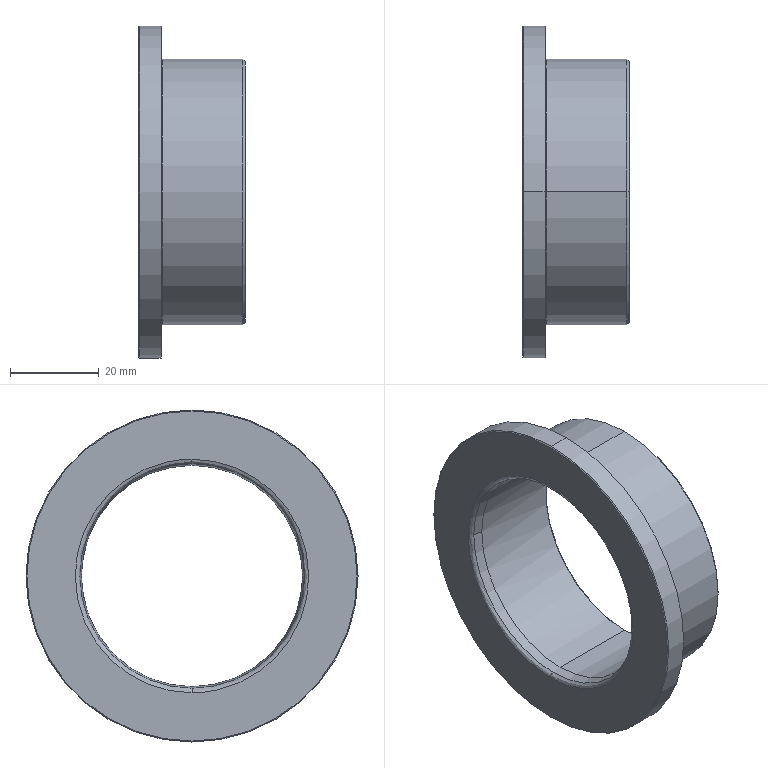Part | SolidWorks | features BaseBody 1, Chamfer 1, ICE 1 | 1 solid | 21 faces | box 24 x 75 x 75 mm | volume 28495 mm3 | cone 8 | cylinder 6 | spline 4 | plane 3 | commonest cylinder face diameters 50 x2 60 x2 75 x2
STEP:
#1=CARTESIAN_POINT('',(-10.,0.,30.3));
#2=VERTEX_POINT('',#1);
#3=CARTESIAN_POINT('',(-10.,0.,-30.3));
#4=VERTEX_POINT('',#3);
#5=CARTESIAN_POINT('',(-10.,0.,30.3));
#6=CARTESIAN_POINT('',(-10.,0.9265,30.3));
#7=CARTESIAN_POINT('',(-10.,2.311,30.237));
#8=CARTESIAN_POINT('',(-10.,3.915,30.052));
#9=CARTESIAN_POINT('',(-10.,4.715,29.932));
#10=CARTESIAN_POINT('',(-10.,5.115,29.866));
#11=CARTESIAN_POINT('',(-10.,5.314,29.83));
#12=CARTESIAN_POINT('',(-10.,5.4,29.815));
#13=CARTESIAN_POINT('',(-10.,5.457,29.805));
#14=CARTESIAN_POINT('',(-10.,5.483,29.8));
#15=CARTESIAN_POINT('',(-10.,6.48,29.615));
#16=CARTESIAN_POINT('',(-10.,7.909,29.279));
#17=CARTESIAN_POINT('',(-10.,9.543,28.766));
#18=CARTESIAN_POINT('',(-10.,10.351,28.479));
#19=CARTESIAN_POINT('',(-10.,10.753,28.328));
#20=CARTESIAN_POINT('',(-10.,10.953,28.251));
#21=CARTESIAN_POINT('',(-10.,11.039,28.218));
#22=CARTESIAN_POINT('',(-10.,11.096,28.195));
#23=CARTESIAN_POINT('',(-10.,11.124,28.184));
#24=CARTESIAN_POINT('',(-10.,12.105,27.796));
#25=CARTESIAN_POINT('',(-10.,13.497,27.162));
#26=CARTESIAN_POINT('',(-10.,15.06,26.301));
#27=CARTESIAN_POINT('',(-10.,15.825,25.841));
#28=CARTESIAN_POINT('',(-10.,16.204,25.604));
#29=CARTESIAN_POINT('',(-10.,16.366,25.5));
#30=CARTESIAN_POINT('',(-10.,16.473,25.431));
#31=CARTESIAN_POINT('',(-10.,16.526,25.397));
#32=CARTESIAN_POINT('',(-10.,18.331,24.217));
#33=CARTESIAN_POINT('',(-10.,19.946,22.904));
#34=CARTESIAN_POINT('',(-10.,22.165,20.686));
#35=CARTESIAN_POINT('',(-10.,23.211,19.526));
#36=CARTESIAN_POINT('',(-10.,24.323,18.083));
#37=CARTESIAN_POINT('',(-10.,24.851,17.339));
#38=CARTESIAN_POINT('',(-10.,25.108,16.962));
#39=CARTESIAN_POINT('',(-10.,25.217,16.799));
#40=CARTESIAN_POINT('',(-10.,25.289,16.69));
#41=CARTESIAN_POINT('',(-10.,25.326,16.634));
#42=CARTESIAN_POINT('',(-10.,25.921,15.724));
#43=CARTESIAN_POINT('',(-10.,26.693,14.403));
#44=CARTESIAN_POINT('',(-10.,27.473,12.799));
#45=CARTESIAN_POINT('',(-10.,27.833,11.981));
#46=CARTESIAN_POINT('',(-10.,28.005,11.569));
#47=CARTESIAN_POINT('',(-10.,28.089,11.361));
#48=CARTESIAN_POINT('',(-10.,28.125,11.272));
#49=CARTESIAN_POINT('',(-10.,28.149,11.213));
#50=CARTESIAN_POINT('',(-10.,28.161,11.182));
#51=CARTESIAN_POINT('',(-10.,28.534,10.24));
#52=CARTESIAN_POINT('',(-10.,29.008,8.85));
#53=CARTESIAN_POINT('',(-10.,29.441,7.193));
#54=CARTESIAN_POINT('',(-10.,29.628,6.356));
#55=CARTESIAN_POINT('',(-10.,29.713,5.936));
#56=CARTESIAN_POINT('',(-10.,29.754,5.725));
#57=CARTESIAN_POINT('',(-10.,29.772,5.634));
#58=CARTESIAN_POINT('',(-10.,29.783,5.574));
#59=CARTESIAN_POINT('',(-10.,29.789,5.542));
#60=CARTESIAN_POINT('',(-10.,30.131,3.691));
#61=CARTESIAN_POINT('',(-10.,30.3,1.853));
#62=CARTESIAN_POINT('',(-10.,30.3,-0.9265));
#63=CARTESIAN_POINT('',(-10.,30.237,-2.311));
#64=CARTESIAN_POINT('',(-10.,30.052,-3.915));
#65=CARTESIAN_POINT('',(-10.,29.932,-4.715));
#66=CARTESIAN_POINT('',(-10.,29.866,-5.115));
#67=CARTESIAN_POINT('',(-10.,29.83,-5.314));
#68=CARTESIAN_POINT('',(-10.,29.815,-5.4));
#69=CARTESIAN_POINT('',(-10.,29.805,-5.457));
#70=CARTESIAN_POINT('',(-10.,29.8,-5.483));
#71=CARTESIAN_POINT('',(-10.,29.615,-6.48));
#72=CARTESIAN_POINT('',(-10.,29.279,-7.909));
#73=CARTESIAN_POINT('',(-10.,28.766,-9.543));
#74=CARTESIAN_POINT('',(-10.,28.479,-10.351));
#75=CARTESIAN_POINT('',(-10.,28.328,-10.753));
#76=CARTESIAN_POINT('',(-10.,28.251,-10.953));
#77=CARTESIAN_POINT('',(-10.,28.218,-11.039));
#78=CARTESIAN_POINT('',(-10.,28.195,-11.096));
#79=CARTESIAN_POINT('',(-10.,28.184,-11.124));
#80=CARTESIAN_POINT('',(-10.,27.796,-12.105));
#81=CARTESIAN_POINT('',(-10.,27.162,-13.497));
#82=CARTESIAN_POINT('',(-10.,26.301,-15.06));
#83=CARTESIAN_POINT('',(-10.,25.841,-15.825));
#84=CARTESIAN_POINT('',(-10.,25.604,-16.204));
#85=CARTESIAN_POINT('',(-10.,25.5,-16.366));
#86=CARTESIAN_POINT('',(-10.,25.431,-16.473));
#87=CARTESIAN_POINT('',(-10.,25.397,-16.526));
#88=CARTESIAN_POINT('',(-10.,24.217,-18.331));
#89=CARTESIAN_POINT('',(-10.,22.904,-19.946));
#90=CARTESIAN_POINT('',(-10.,20.686,-22.165));
#91=CARTESIAN_POINT('',(-10.,19.526,-23.211));
#92=CARTESIAN_POINT('',(-10.,18.083,-24.323));
#93=CARTESIAN_POINT('',(-10.,17.339,-24.851));
#94=CARTESIAN_POINT('',(-10.,16.962,-25.108));
#95=CARTESIAN_POINT('',(-10.,16.799,-25.217));
#96=CARTESIAN_POINT('',(-10.,16.69,-25.289));
#97=CARTESIAN_POINT('',(-10.,16.634,-25.326));
#98=CARTESIAN_POINT('',(-10.,15.724,-25.921));
#99=CARTESIAN_POINT('',(-10.,14.403,-26.693));
#100=CARTESIAN_POINT('',(-10.,12.799,-27.473));
#101=CARTESIAN_POINT('',(-10.,11.981,-27.833));
#102=CARTESIAN_POINT('',(-10.,11.569,-28.005));
#103=CARTESIAN_POINT('',(-10.,11.361,-28.089));
#104=CARTESIAN_POINT('',(-10.,11.272,-28.125));
#105=CARTESIAN_POINT('',(-10.,11.213,-28.149));
#106=CARTESIAN_POINT('',(-10.,11.182,-28.161));
#107=CARTESIAN_POINT('',(-10.,10.24,-28.534));
#108=CARTESIAN_POINT('',(-10.,8.85,-29.008));
#109=CARTESIAN_POINT('',(-10.,7.193,-29.441));
#110=CARTESIAN_POINT('',(-10.,6.356,-29.628));
#111=CARTESIAN_POINT('',(-10.,5.936,-29.713));
#112=CARTESIAN_POINT('',(-10.,5.725,-29.754));
#113=CARTESIAN_POINT('',(-10.,5.634,-29.772));
#114=CARTESIAN_POINT('',(-10.,5.574,-29.783));
#115=CARTESIAN_POINT('',(-10.,5.542,-29.789));
#116=CARTESIAN_POINT('',(-10.,3.691,-30.131));
#117=CARTESIAN_POINT('',(-10.,1.853,-30.3));
#118=CARTESIAN_POINT('',(-10.,0.,-30.3));
#119=B_SPLINE_CURVE_WITH_KNOTS('',3,(#5,#6,#7,#8,#9,#10,#11,#12,#13,#14,#15,#16,#17,#18,#19,#20,#21,#22,#23,#24,#25,#26,#27,#28,#29,#30,#31,#32,#33,#34,#35,#36,#37,#38,#39,#40,#41,#42,#43,#44,#45,#46,#47,#48,#49,#50,#51,#52,#53,#54,#55,#56,#57,#58,#59,#60,#61,#62,#63,#64,#65,#66,#67,#68,#69,#70,#71,#72,#73,#74,#75,#76,#77,#78,#79,#80,#81,#82,#83,#84,#85,#86,#87,#88,#89,#90,#91,#92,#93,#94,#95,#96,#97,#98,#99,#100,#101,#102,#103,#104,#105,#106,#107,#108,#109,#110,#111,#112,#113,#114,#115,#116,#117,#118),.UNSPECIFIED.,.F.,.F.,(4,1,1,1,1,1,2,2,1,1,1,1,1,2,2,1,1,1,1,2,2,2,1,1,1,1,2,2,1,1,1,1,1,2,2,1,1,1,1,1,2,2,2,1,1,1,1,1,2,2,1,1,1,1,1,2,2,1,1,1,1,2,2,2,1,1,1,1,2,2,1,1,1,1,1,2,2,1,1,1,1,1,2,2,4),(0.5,0.5156,0.5234,0.5273,0.5293,0.5303,0.5308,0.5313,0.5469,0.5547,0.5586,0.5605,0.5615,0.562,0.5625,0.5781,0.5859,0.5898,0.5918,0.5928,0.5938,0.625,0.6406,0.6484,0.6523,0.6543,0.6553,0.6562,0.6719,0.6797,0.6836,0.6855,0.6865,0.687,0.6875,0.7031,0.7109,0.7148,0.7168,0.7178,0.7183,0.7188,0.75,0.7656,0.7734,0.7773,0.7793,0.7803,0.7808,0.7813,0.7969,0.8047,0.8086,0.8105,0.8115,0.812,0.8125,0.8281,0.8359,0.8398,0.8418,0.8428,0.8438,0.875,0.8906,0.8984,0.9023,0.9043,0.9053,0.9062,0.9219,0.9297,0.9336,0.9355,0.9365,0.937,0.9375,0.9531,0.9609,0.9648,0.9668,0.9678,0.9683,0.9688,1.),.UNSPECIFIED.);
#120=EDGE_CURVE('',#2,#4,#119,.T.);
#121=ORIENTED_EDGE('',*,*,#120,.F.);
#122=CARTESIAN_POINT('',(-9.7,0.,30.));
#123=VERTEX_POINT('',#122);
#124=CARTESIAN_POINT('',(-9.7,0.,30.3));
#125=DIRECTION('',(0.,-1.,0.));
#126=DIRECTION('',(0.,0.,1.));
#127=AXIS2_PLACEMENT_3D('',#124,#125,#126);
#128=CIRCLE('',#127,0.3);
#129=EDGE_CURVE('',#2,#123,#128,.T.);
#130=ORIENTED_EDGE('',*,*,#129,.T.);
#131=CARTESIAN_POINT('',(-9.7,0.,-30.));
#132=VERTEX_POINT('',#131);
#133=CARTESIAN_POINT('',(-9.7,0.,0.));
#134=DIRECTION('',(1.,0.,0.));
#135=DIRECTION('',(0.,0.,1.));
#136=AXIS2_PLACEMENT_3D('',#133,#134,#135);
#137=CIRCLE('',#136,30.);
#138=EDGE_CURVE('',#132,#123,#137,.T.);
#139=ORIENTED_EDGE('',*,*,#138,.F.);
#140=CARTESIAN_POINT('',(-9.7,0.,-30.3));
#141=DIRECTION('',(0.,1.,0.));
#142=DIRECTION('',(0.,0.,-1.));
#143=AXIS2_PLACEMENT_3D('',#140,#141,#142);
#144=CIRCLE('',#143,0.3);
#145=EDGE_CURVE('',#4,#132,#144,.T.);
#146=ORIENTED_EDGE('',*,*,#145,.F.);
#147=EDGE_LOOP('',(#121,#130,#139,#146));
#148=FACE_OUTER_BOUND('',#147,.T.);
#149=CARTESIAN_POINT('',(-10.,0.,-30.3));
#150=CARTESIAN_POINT('',(-10.,60.6,-30.3));
#151=CARTESIAN_POINT('',(-10.,60.6,30.3));
#152=CARTESIAN_POINT('',(-10.,0.,30.3));
#153=CARTESIAN_POINT('',(-10.,0.,-30.124));
#154=CARTESIAN_POINT('',(-10.,60.249,-30.124));
#155=CARTESIAN_POINT('',(-10.,60.249,30.124));
#156=CARTESIAN_POINT('',(-10.,0.,30.124));
#157=CARTESIAN_POINT('',(-9.876,0.,-30.));
#158=CARTESIAN_POINT('',(-9.876,60.,-30.));
#159=CARTESIAN_POINT('',(-9.876,60.,30.));
#160=CARTESIAN_POINT('',(-9.876,0.,30.));
#161=CARTESIAN_POINT('',(-9.7,0.,-30.));
#162=CARTESIAN_POINT('',(-9.7,60.,-30.));
#163=CARTESIAN_POINT('',(-9.7,60.,30.));
#164=CARTESIAN_POINT('',(-9.7,0.,30.));
#165=(BOUNDED_SURFACE()B_SPLINE_SURFACE(3,3,((#149,#150,#151,#152),(#153,#154,#155,#156),(#157,#158,#159,#160),(#161,#162,#163,#164)),.UNSPECIFIED.,.F.,.F.,.T.)B_SPLINE_SURFACE_WITH_KNOTS((4,4),(4,4),(0.,1.),(0.,1.),.UNSPECIFIED.)GEOMETRIC_REPRESENTATION_ITEM()RATIONAL_B_SPLINE_SURFACE(((1.,0.3333,0.3333,1.),(0.8047,0.2682,0.2682,0.8047),(0.8047,0.2682,0.2682,0.8047),(1.,0.3333,0.3333,1.)))REPRESENTATION_ITEM('')SURFACE());
#166=ADVANCED_FACE('',(#148),#165,.F.);
#167=CARTESIAN_POINT('',(-15.,0.,26.368));
#168=VERTEX_POINT('',#167);
#169=CARTESIAN_POINT('',(-15.,0.,-26.368));
#170=VERTEX_POINT('',#169);
#171=CARTESIAN_POINT('',(-15.,0.,26.368));
#172=CARTESIAN_POINT('',(-15.,-0.8062,26.368));
#173=CARTESIAN_POINT('',(-15.,-2.011,26.313));
#174=CARTESIAN_POINT('',(-15.,-3.407,26.153));
#175=CARTESIAN_POINT('',(-15.,-4.103,26.048));
#176=CARTESIAN_POINT('',(-15.,-4.451,25.99));
#177=CARTESIAN_POINT('',(-15.,-4.624,25.959));
#178=CARTESIAN_POINT('',(-15.,-4.699,25.946));
#179=CARTESIAN_POINT('',(-15.,-4.748,25.937));
#180=CARTESIAN_POINT('',(-15.,-4.772,25.933));
#181=CARTESIAN_POINT('',(-15.,-5.639,25.772));
#182=CARTESIAN_POINT('',(-15.,-6.883,25.479));
#183=CARTESIAN_POINT('',(-15.,-8.304,25.033));
#184=CARTESIAN_POINT('',(-15.,-9.008,24.783));
#185=CARTESIAN_POINT('',(-15.,-9.357,24.652));
#186=CARTESIAN_POINT('',(-15.,-9.507,24.595));
#187=CARTESIAN_POINT('',(-15.,-9.606,24.556));
#188=CARTESIAN_POINT('',(-15.,-9.654,24.537));
#189=CARTESIAN_POINT('',(-15.,-10.534,24.189));
#190=CARTESIAN_POINT('',(-15.,-11.746,23.637));
#191=CARTESIAN_POINT('',(-15.,-13.105,22.888));
#192=CARTESIAN_POINT('',(-15.,-13.772,22.488));
#193=CARTESIAN_POINT('',(-15.,-14.101,22.281));
#194=CARTESIAN_POINT('',(-15.,-14.242,22.191));
#195=CARTESIAN_POINT('',(-15.,-14.336,22.131));
#196=CARTESIAN_POINT('',(-15.,-14.381,22.101));
#197=CARTESIAN_POINT('',(-15.,-15.952,21.074));
#198=CARTESIAN_POINT('',(-15.,-17.358,19.932));
#199=CARTESIAN_POINT('',(-15.,-19.289,18.002));
#200=CARTESIAN_POINT('',(-15.,-20.199,16.992));
#201=CARTESIAN_POINT('',(-15.,-21.166,15.736));
#202=CARTESIAN_POINT('',(-15.,-21.626,15.089));
#203=CARTESIAN_POINT('',(-15.,-21.85,14.761));
#204=CARTESIAN_POINT('',(-15.,-21.945,14.619));
#205=CARTESIAN_POINT('',(-15.,-22.008,14.524));
#206=CARTESIAN_POINT('',(-15.,-22.039,14.475));
#207=CARTESIAN_POINT('',(-15.,-22.557,13.683));
#208=CARTESIAN_POINT('',(-15.,-23.229,12.534));
#209=CARTESIAN_POINT('',(-15.,-23.908,11.138));
#210=CARTESIAN_POINT('',(-15.,-24.221,10.426));
#211=CARTESIAN_POINT('',(-15.,-24.371,10.067));
#212=CARTESIAN_POINT('',(-15.,-24.444,9.887));
#213=CARTESIAN_POINT('',(-15.,-24.476,9.809));
#214=CARTESIAN_POINT('',(-15.,-24.496,9.758));
#215=CARTESIAN_POINT('',(-15.,-24.507,9.731));
#216=CARTESIAN_POINT('',(-15.,-24.831,8.911));
#217=CARTESIAN_POINT('',(-15.,-25.244,7.701));
#218=CARTESIAN_POINT('',(-15.,-25.621,6.26));
#219=CARTESIAN_POINT('',(-15.,-25.783,5.531));
#220=CARTESIAN_POINT('',(-15.,-25.858,5.165));
#221=CARTESIAN_POINT('',(-15.,-25.893,4.982));
#222=CARTESIAN_POINT('',(-15.,-25.908,4.903));
#223=CARTESIAN_POINT('',(-15.,-25.918,4.851));
#224=CARTESIAN_POINT('',(-15.,-25.923,4.823));
#225=CARTESIAN_POINT('',(-15.,-26.221,3.212));
#226=CARTESIAN_POINT('',(-15.,-26.368,1.612));
#227=CARTESIAN_POINT('',(-15.,-26.368,-0.8062));
#228=CARTESIAN_POINT('',(-15.,-26.313,-2.011));
#229=CARTESIAN_POINT('',(-15.,-26.153,-3.407));
#230=CARTESIAN_POINT('',(-15.,-26.048,-4.103));
#231=CARTESIAN_POINT('',(-15.,-25.99,-4.451));
#232=CARTESIAN_POINT('',(-15.,-25.959,-4.624));
#233=CARTESIAN_POINT('',(-15.,-25.946,-4.699));
#234=CARTESIAN_POINT('',(-15.,-25.937,-4.748));
#235=CARTESIAN_POINT('',(-15.,-25.933,-4.772));
#236=CARTESIAN_POINT('',(-15.,-25.772,-5.639));
#237=CARTESIAN_POINT('',(-15.,-25.479,-6.883));
#238=CARTESIAN_POINT('',(-15.,-25.033,-8.304));
#239=CARTESIAN_POINT('',(-15.,-24.783,-9.008));
#240=CARTESIAN_POINT('',(-15.,-24.652,-9.357));
#241=CARTESIAN_POINT('',(-15.,-24.595,-9.507));
#242=CARTESIAN_POINT('',(-15.,-24.556,-9.606));
#243=CARTESIAN_POINT('',(-15.,-24.537,-9.654));
#244=CARTESIAN_POINT('',(-15.,-24.189,-10.534));
#245=CARTESIAN_POINT('',(-15.,-23.637,-11.746));
#246=CARTESIAN_POINT('',(-15.,-22.888,-13.105));
#247=CARTESIAN_POINT('',(-15.,-22.488,-13.772));
#248=CARTESIAN_POINT('',(-15.,-22.281,-14.101));
#249=CARTESIAN_POINT('',(-15.,-22.191,-14.242));
#250=CARTESIAN_POINT('',(-15.,-22.131,-14.336));
#251=CARTESIAN_POINT('',(-15.,-22.101,-14.381));
#252=CARTESIAN_POINT('',(-15.,-21.074,-15.952));
#253=CARTESIAN_POINT('',(-15.,-19.932,-17.358));
#254=CARTESIAN_POINT('',(-15.,-18.002,-19.289));
#255=CARTESIAN_POINT('',(-15.,-16.992,-20.199));
#256=CARTESIAN_POINT('',(-15.,-15.736,-21.166));
#257=CARTESIAN_POINT('',(-15.,-15.089,-21.626));
#258=CARTESIAN_POINT('',(-15.,-14.761,-21.85));
#259=CARTESIAN_POINT('',(-15.,-14.619,-21.945));
#260=CARTESIAN_POINT('',(-15.,-14.524,-22.008));
#261=CARTESIAN_POINT('',(-15.,-14.475,-22.039));
#262=CARTESIAN_POINT('',(-15.,-13.683,-22.557));
#263=CARTESIAN_POINT('',(-15.,-12.534,-23.229));
#264=CARTESIAN_POINT('',(-15.,-11.138,-23.908));
#265=CARTESIAN_POINT('',(-15.,-10.426,-24.221));
#266=CARTESIAN_POINT('',(-15.,-10.067,-24.371));
#267=CARTESIAN_POINT('',(-15.,-9.887,-24.444));
#268=CARTESIAN_POINT('',(-15.,-9.809,-24.476));
#269=CARTESIAN_POINT('',(-15.,-9.758,-24.496));
#270=CARTESIAN_POINT('',(-15.,-9.731,-24.507));
#271=CARTESIAN_POINT('',(-15.,-8.911,-24.831));
#272=CARTESIAN_POINT('',(-15.,-7.701,-25.244));
#273=CARTESIAN_POINT('',(-15.,-6.26,-25.621));
#274=CARTESIAN_POINT('',(-15.,-5.531,-25.783));
#275=CARTESIAN_POINT('',(-15.,-5.165,-25.858));
#276=CARTESIAN_POINT('',(-15.,-4.982,-25.893));
#277=CARTESIAN_POINT('',(-15.,-4.903,-25.908));
#278=CARTESIAN_POINT('',(-15.,-4.851,-25.918));
#279=CARTESIAN_POINT('',(-15.,-4.823,-25.923));
#280=CARTESIAN_POINT('',(-15.,-3.212,-26.221));
#281=CARTESIAN_POINT('',(-15.,-1.613,-26.368));
#282=CARTESIAN_POINT('',(-15.,0.,-26.368));
#283=B_SPLINE_CURVE_WITH_KNOTS('',3,(#171,#172,#173,#174,#175,#176,#177,#178,#179,#180,#181,#182,#183,#184,#185,#186,#187,#188,#189,#190,#191,#192,#193,#194,#195,#196,#197,#198,#199,#200,#201,#202,#203,#204,#205,#206,#207,#208,#209,#210,#211,#212,#213,#214,#215,#216,#217,#218,#219,#220,#221,#222,#223,#224,#225,#226,#227,#228,#229,#230,#231,#232,#233,#234,#235,#236,#237,#238,#239,#240,#241,#242,#243,#244,#245,#246,#247,#248,#249,#250,#251,#252,#253,#254,#255,#256,#257,#258,#259,#260,#261,#262,#263,#264,#265,#266,#267,#268,#269,#270,#271,#272,#273,#274,#275,#276,#277,#278,#279,#280,#281,#282),.UNSPECIFIED.,.F.,.F.,(4,1,1,1,1,1,2,2,1,1,1,1,2,2,1,1,1,1,2,2,2,1,1,1,1,2,2,1,1,1,1,1,2,2,1,1,1,1,1,2,2,2,1,1,1,1,1,2,2,1,1,1,1,2,2,1,1,1,1,2,2,2,1,1,1,1,2,2,1,1,1,1,1,2,2,1,1,1,1,1,2,2,4),(0.5,0.5156,0.5234,0.5273,0.5293,0.5303,0.5308,0.5313,0.5469,0.5547,0.5586,0.5605,0.5615,0.5625,0.5781,0.5859,0.5898,0.5918,0.5928,0.5938,0.625,0.6406,0.6484,0.6523,0.6543,0.6553,0.6563,0.6719,0.6797,0.6836,0.6855,0.6865,0.687,0.6875,0.7031,0.7109,0.7148,0.7168,0.7178,0.7183,0.7188,0.75,0.7656,0.7734,0.7773,0.7793,0.7803,0.7808,0.7813,0.7969,0.8047,0.8086,0.8105,0.8115,0.8125,0.8281,0.8359,0.8398,0.8418,0.8428,0.8438,0.875,0.8906,0.8984,0.9023,0.9043,0.9053,0.9063,0.9219,0.9297,0.9336,0.9355,0.9365,0.937,0.9375,0.9531,0.9609,0.9648,0.9668,0.9678,0.9683,0.9688,1.),.UNSPECIFIED.);
#284=EDGE_CURVE('',#168,#170,#283,.T.);
#285=ORIENTED_EDGE('',*,*,#284,.F.);
#286=CARTESIAN_POINT('',(-14.174,0.,25.383));
#287=VERTEX_POINT('',#286);
#288=CARTESIAN_POINT('',(-14.,0.,26.368));
#289=DIRECTION('',(0.,-1.,0.));
#290=DIRECTION('',(0.,0.,1.));
#291=AXIS2_PLACEMENT_3D('',#288,#289,#290);
#292=CIRCLE('',#291,1.);
#293=EDGE_CURVE('',#168,#287,#292,.T.);
#294=ORIENTED_EDGE('',*,*,#293,.T.);
#295=CARTESIAN_POINT('',(-14.174,-25.383,0.));
#296=VERTEX_POINT('',#295);
#297=CARTESIAN_POINT('',(-14.174,0.,0.));
#298=DIRECTION('',(1.,0.,0.));
#299=DIRECTION('',(0.,0.,1.));
#300=AXIS2_PLACEMENT_3D('',#297,#298,#299);
#301=CIRCLE('',#300,25.383);
#302=EDGE_CURVE('',#287,#296,#301,.T.);
#303=ORIENTED_EDGE('',*,*,#302,.T.);
#304=CARTESIAN_POINT('',(-14.174,0.,-25.383));
#305=VERTEX_POINT('',#304);
#306=CARTESIAN_POINT('',(-14.174,0.,0.));
#307=DIRECTION('',(1.,0.,0.));
#308=DIRECTION('',(0.,0.,1.));
#309=AXIS2_PLACEMENT_3D('',#306,#307,#308);
#310=CIRCLE('',#309,25.383);
#311=EDGE_CURVE('',#296,#305,#310,.T.);
#312=ORIENTED_EDGE('',*,*,#311,.T.);
#313=CARTESIAN_POINT('',(-14.,0.,-26.368));
#314=DIRECTION('',(0.,1.,0.));
#315=DIRECTION('',(0.,0.,-1.));
#316=AXIS2_PLACEMENT_3D('',#313,#314,#315);
#317=CIRCLE('',#316,1.);
#318=EDGE_CURVE('',#170,#305,#317,.T.);
#319=ORIENTED_EDGE('',*,*,#318,.F.);
#320=EDGE_LOOP('',(#285,#294,#303,#312,#319));
#321=FACE_OUTER_BOUND('',#320,.T.);
#322=CARTESIAN_POINT('',(-15.,0.,26.368));
#323=CARTESIAN_POINT('',(-15.,-52.736,26.368));
#324=CARTESIAN_POINT('',(-15.,-52.736,-26.368));
#325=CARTESIAN_POINT('',(-15.,0.,-26.368));
#326=CARTESIAN_POINT('',(-15.,0.,25.86));
#327=CARTESIAN_POINT('',(-15.,-51.721,25.86));
#328=CARTESIAN_POINT('',(-15.,-51.721,-25.86));
#329=CARTESIAN_POINT('',(-15.,0.,-25.86));
#330=CARTESIAN_POINT('',(-14.674,0.,25.471));
#331=CARTESIAN_POINT('',(-14.674,-50.943,25.471));
#332=CARTESIAN_POINT('',(-14.674,-50.943,-25.471));
#333=CARTESIAN_POINT('',(-14.674,0.,-25.471));
#334=CARTESIAN_POINT('',(-14.174,0.,25.383));
#335=CARTESIAN_POINT('',(-14.174,-50.767,25.383));
#336=CARTESIAN_POINT('',(-14.174,-50.767,-25.383));
#337=CARTESIAN_POINT('',(-14.174,0.,-25.383));
#338=(BOUNDED_SURFACE()B_SPLINE_SURFACE(3,3,((#322,#323,#324,#325),(#326,#327,#328,#329),(#330,#331,#332,#333),(#334,#335,#336,#337)),.UNSPECIFIED.,.F.,.F.,.T.)B_SPLINE_SURFACE_WITH_KNOTS((4,4),(4,4),(0.,1.),(0.,1.),.UNSPECIFIED.)GEOMETRIC_REPRESENTATION_ITEM()RATIONAL_B_SPLINE_SURFACE(((1.,0.3333,0.3333,1.),(0.844,0.2813,0.2813,0.844),(0.844,0.2813,0.2813,0.844),(1.,0.3333,0.3333,1.)))REPRESENTATION_ITEM('')SURFACE());
#339=ADVANCED_FACE('',(#321),#338,.T.);
#340=CARTESIAN_POINT('',(8.5,0.,25.));
#341=VERTEX_POINT('',#340);
#342=CARTESIAN_POINT('',(8.5,0.,-25.));
#343=VERTEX_POINT('',#342);
#344=CARTESIAN_POINT('',(8.5,0.,0.));
#345=DIRECTION('',(1.,0.,0.));
#346=DIRECTION('',(0.,0.,-1.));
#347=AXIS2_PLACEMENT_3D('',#344,#345,#346);
#348=CIRCLE('',#347,25.);
#349=EDGE_CURVE('',#341,#343,#348,.T.);
#350=ORIENTED_EDGE('',*,*,#349,.F.);
#351=CARTESIAN_POINT('',(9.,0.,25.5));
#352=VERTEX_POINT('',#351);
#353=CARTESIAN_POINT('',(9.,0.,25.5));
#354=DIRECTION('',(0.7071,0.,0.7071));
#355=VECTOR('',#354,1000.);
#356=LINE('',#353,#355);
#357=EDGE_CURVE('',#341,#352,#356,.T.);
#358=ORIENTED_EDGE('',*,*,#357,.T.);
#359=CARTESIAN_POINT('',(9.,0.,-25.5));
#360=VERTEX_POINT('',#359);
#361=CARTESIAN_POINT('',(9.,0.,0.));
#362=DIRECTION('',(-1.,0.,0.));
#363=DIRECTION('',(0.,0.,-1.));
#364=AXIS2_PLACEMENT_3D('',#361,#362,#363);
#365=CIRCLE('',#364,25.5);
#366=EDGE_CURVE('',#360,#352,#365,.T.);
#367=ORIENTED_EDGE('',*,*,#366,.F.);
#368=CARTESIAN_POINT('',(9.,0.,-25.5));
#369=DIRECTION('',(0.7071,0.,-0.7071));
#370=VECTOR('',#369,1000.);
#371=LINE('',#368,#370);
#372=EDGE_CURVE('',#343,#360,#371,.T.);
#373=ORIENTED_EDGE('',*,*,#372,.F.);
#374=EDGE_LOOP('',(#350,#358,#367,#373));
#375=FACE_OUTER_BOUND('',#374,.T.);
#376=CARTESIAN_POINT('',(9.,0.,0.));
#377=DIRECTION('',(1.,0.,0.));
#378=DIRECTION('',(0.,0.,-1.));
#379=AXIS2_PLACEMENT_3D('',#376,#377,#378);
#380=CONICAL_SURFACE('',#379,25.5,0.7854);
#381=ADVANCED_FACE('',(#375),#380,.F.);
#382=CARTESIAN_POINT('',(9.,0.,-29.5));
#383=VERTEX_POINT('',#382);
#384=CARTESIAN_POINT('',(9.,0.,29.5));
#385=VERTEX_POINT('',#384);
#386=CARTESIAN_POINT('',(9.,0.,0.));
#387=DIRECTION('',(1.,0.,0.));
#388=DIRECTION('',(0.,0.,-1.));
#389=AXIS2_PLACEMENT_3D('',#386,#387,#388);
#390=CIRCLE('',#389,29.5);
#391=EDGE_CURVE('',#383,#385,#390,.T.);
#392=ORIENTED_EDGE('',*,*,#391,.F.);
#393=CARTESIAN_POINT('',(8.5,0.,-30.));
#394=VERTEX_POINT('',#393);
#395=CARTESIAN_POINT('',(8.5,0.,-30.));
#396=DIRECTION('',(-0.7071,0.,-0.7071));
#397=VECTOR('',#396,1000.);
#398=LINE('',#395,#397);
#399=EDGE_CURVE('',#383,#394,#398,.T.);
#400=ORIENTED_EDGE('',*,*,#399,.T.);
#401=CARTESIAN_POINT('',(8.5,0.,30.));
#402=VERTEX_POINT('',#401);
#403=CARTESIAN_POINT('',(8.5,0.,0.));
#404=DIRECTION('',(-1.,0.,0.));
#405=DIRECTION('',(0.,0.,-1.));
#406=AXIS2_PLACEMENT_3D('',#403,#404,#405);
#407=CIRCLE('',#406,30.);
#408=EDGE_CURVE('',#402,#394,#407,.T.);
#409=ORIENTED_EDGE('',*,*,#408,.F.);
#410=CARTESIAN_POINT('',(8.5,0.,30.));
#411=DIRECTION('',(-0.7071,0.,0.7071));
#412=VECTOR('',#411,1000.);
#413=LINE('',#410,#412);
#414=EDGE_CURVE('',#385,#402,#413,.T.);
#415=ORIENTED_EDGE('',*,*,#414,.F.);
#416=EDGE_LOOP('',(#392,#400,#409,#415));
#417=FACE_OUTER_BOUND('',#416,.T.);
#418=CARTESIAN_POINT('',(8.5,0.,0.));
#419=DIRECTION('',(-1.,0.,0.));
#420=DIRECTION('',(0.,0.,1.));
#421=AXIS2_PLACEMENT_3D('',#418,#419,#420);
#422=CONICAL_SURFACE('',#421,30.,0.7854);
#423=ADVANCED_FACE('',(#417),#422,.T.);
#424=CARTESIAN_POINT('',(-10.,0.,-37.5));
#425=VERTEX_POINT('',#424);
#426=CARTESIAN_POINT('',(-10.,0.,37.5));
#427=VERTEX_POINT('',#426);
#428=CARTESIAN_POINT('',(-10.,0.,0.));
#429=DIRECTION('',(1.,0.,0.));
#430=DIRECTION('',(0.,0.,1.));
#431=AXIS2_PLACEMENT_3D('',#428,#429,#430);
#432=CIRCLE('',#431,37.5);
#433=EDGE_CURVE('',#425,#427,#432,.T.);
#434=ORIENTED_EDGE('',*,*,#433,.F.);
#435=CARTESIAN_POINT('',(-14.788,0.,-37.5));
#436=VERTEX_POINT('',#435);
#437=CARTESIAN_POINT('',(20.,0.,-37.5));
#438=DIRECTION('',(-1.,0.,0.));
#439=VECTOR('',#438,1000.);
#440=LINE('',#437,#439);
#441=EDGE_CURVE('',#425,#436,#440,.T.);
#442=ORIENTED_EDGE('',*,*,#441,.T.);
#443=CARTESIAN_POINT('',(-14.788,37.5,0.));
#444=VERTEX_POINT('',#443);
#445=CARTESIAN_POINT('',(-14.788,0.,0.));
#446=DIRECTION('',(1.,0.,0.));
#447=DIRECTION('',(0.,0.,1.));
#448=AXIS2_PLACEMENT_3D('',#445,#446,#447);
#449=CIRCLE('',#448,37.5);
#450=EDGE_CURVE('',#436,#444,#449,.T.);
#451=ORIENTED_EDGE('',*,*,#450,.T.);
#452=CARTESIAN_POINT('',(-14.788,0.,37.5));
#453=VERTEX_POINT('',#452);
#454=CARTESIAN_POINT('',(-14.788,0.,0.));
#455=DIRECTION('',(1.,0.,0.));
#456=DIRECTION('',(0.,0.,1.));
#457=AXIS2_PLACEMENT_3D('',#454,#455,#456);
#458=CIRCLE('',#457,37.5);
#459=EDGE_CURVE('',#444,#453,#458,.T.);
#460=ORIENTED_EDGE('',*,*,#459,.T.);
#461=CARTESIAN_POINT('',(20.,0.,37.5));
#462=DIRECTION('',(-1.,0.,0.));
#463=VECTOR('',#462,1000.);
#464=LINE('',#461,#463);
#465=EDGE_CURVE('',#427,#453,#464,.T.);
#466=ORIENTED_EDGE('',*,*,#465,.F.);
#467=EDGE_LOOP('',(#434,#442,#451,#460,#466));
#468=FACE_OUTER_BOUND('',#467,.T.);
#469=CARTESIAN_POINT('',(20.,0.,0.));
#470=DIRECTION('',(-1.,0.,0.));
#471=DIRECTION('',(0.,0.,1.));
#472=AXIS2_PLACEMENT_3D('',#469,#470,#471);
#473=CYLINDRICAL_SURFACE('',#472,37.5);
#474=ADVANCED_FACE('',(#468),#473,.T.);
#475=CARTESIAN_POINT('',(-15.,37.288,0.));
#476=VERTEX_POINT('',#475);
#477=CARTESIAN_POINT('',(-15.,-37.288,0.));
#478=VERTEX_POINT('',#477);
#479=CARTESIAN_POINT('',(-15.,0.,0.));
#480=DIRECTION('',(1.,0.,0.));
#481=DIRECTION('',(0.,1.,0.));
#482=AXIS2_PLACEMENT_3D('',#479,#480,#481);
#483=CIRCLE('',#482,37.288);
#484=EDGE_CURVE('',#476,#478,#483,.T.);
#485=ORIENTED_EDGE('',*,*,#484,.T.);
#486=CARTESIAN_POINT('',(-14.788,-37.5,0.));
#487=VERTEX_POINT('',#486);
#488=CARTESIAN_POINT('',(-14.788,-37.5,0.));
#489=DIRECTION('',(0.7071,-0.7071,0.));
#490=VECTOR('',#489,1000.);
#491=LINE('',#488,#490);
#492=EDGE_CURVE('',#478,#487,#491,.T.);
#493=ORIENTED_EDGE('',*,*,#492,.T.);
#494=CARTESIAN_POINT('',(-14.788,0.,0.));
#495=DIRECTION('',(1.,0.,0.));
#496=DIRECTION('',(0.,0.,1.));
#497=AXIS2_PLACEMENT_3D('',#494,#495,#496);
#498=CIRCLE('',#497,37.5);
#499=EDGE_CURVE('',#453,#487,#498,.T.);
#500=ORIENTED_EDGE('',*,*,#499,.F.);
#501=ORIENTED_EDGE('',*,*,#459,.F.);
#502=CARTESIAN_POINT('',(-14.788,37.5,0.));
#503=DIRECTION('',(0.7071,0.7071,0.));
#504=VECTOR('',#503,1000.);
#505=LINE('',#502,#504);
#506=EDGE_CURVE('',#476,#444,#505,.T.);
#507=ORIENTED_EDGE('',*,*,#506,.F.);
#508=EDGE_LOOP('',(#485,#493,#500,#501,#507));
#509=FACE_OUTER_BOUND('',#508,.T.);
#510=CARTESIAN_POINT('',(-14.788,0.,0.));
#511=DIRECTION('',(1.,0.,0.));
#512=DIRECTION('',(0.,1.,0.));
#513=AXIS2_PLACEMENT_3D('',#510,#511,#512);
#514=CONICAL_SURFACE('',#513,37.5,0.7854);
#515=ADVANCED_FACE('',(#509),#514,.T.);
#516=CARTESIAN_POINT('',(-12.,0.,-25.));
#517=VERTEX_POINT('',#516);
#518=CARTESIAN_POINT('',(-12.,25.,0.));
#519=VERTEX_POINT('',#518);
#520=CARTESIAN_POINT('',(-12.,0.,0.));
#521=DIRECTION('',(1.,0.,0.));
#522=DIRECTION('',(0.,0.,1.));
#523=AXIS2_PLACEMENT_3D('',#520,#521,#522);
#524=CIRCLE('',#523,25.);
#525=EDGE_CURVE('',#517,#519,#524,.T.);
#526=ORIENTED_EDGE('',*,*,#525,.T.);
#527=CARTESIAN_POINT('',(-14.174,25.383,0.));
#528=VERTEX_POINT('',#527);
#529=CARTESIAN_POINT('',(-14.174,25.383,0.));
#530=DIRECTION('',(-0.9848,0.1736,0.));
#531=VECTOR('',#530,1000.);
#532=LINE('',#529,#531);
#533=EDGE_CURVE('',#519,#528,#532,.T.);
#534=ORIENTED_EDGE('',*,*,#533,.T.);
#535=CARTESIAN_POINT('',(-14.174,0.,0.));
#536=DIRECTION('',(1.,0.,0.));
#537=DIRECTION('',(0.,0.,1.));
#538=AXIS2_PLACEMENT_3D('',#535,#536,#537);
#539=CIRCLE('',#538,25.383);
#540=EDGE_CURVE('',#305,#528,#539,.T.);
#541=ORIENTED_EDGE('',*,*,#540,.F.);
#542=ORIENTED_EDGE('',*,*,#311,.F.);
#543=CARTESIAN_POINT('',(-12.,-25.,0.));
#544=VERTEX_POINT('',#543);
#545=CARTESIAN_POINT('',(-14.174,-25.383,0.));
#546=DIRECTION('',(-0.9848,-0.1736,0.));
#547=VECTOR('',#546,1000.);
#548=LINE('',#545,#547);
#549=EDGE_CURVE('',#544,#296,#548,.T.);
#550=ORIENTED_EDGE('',*,*,#549,.F.);
#551=CARTESIAN_POINT('',(-12.,0.,0.));
#552=DIRECTION('',(1.,0.,0.));
#553=DIRECTION('',(0.,0.,1.));
#554=AXIS2_PLACEMENT_3D('',#551,#552,#553);
#555=CIRCLE('',#554,25.);
#556=EDGE_CURVE('',#544,#517,#555,.T.);
#557=ORIENTED_EDGE('',*,*,#556,.T.);
#558=EDGE_LOOP('',(#526,#534,#541,#542,#550,#557));
#559=FACE_OUTER_BOUND('',#558,.T.);
#560=CARTESIAN_POINT('',(-14.174,0.,0.));
#561=DIRECTION('',(-1.,0.,0.));
#562=DIRECTION('',(0.,-1.,0.));
#563=AXIS2_PLACEMENT_3D('',#560,#561,#562);
#564=CONICAL_SURFACE('',#563,25.383,0.1745);
#565=ADVANCED_FACE('',(#559),#564,.F.);
#566=ORIENTED_EDGE('',*,*,#408,.T.);
#567=CARTESIAN_POINT('',(20.,0.,-30.));
#568=DIRECTION('',(-1.,0.,0.));
#569=VECTOR('',#568,1000.);
#570=LINE('',#567,#569);
#571=EDGE_CURVE('',#394,#132,#570,.T.);
#572=ORIENTED_EDGE('',*,*,#571,.T.);
#573=ORIENTED_EDGE('',*,*,#138,.T.);
#574=CARTESIAN_POINT('',(20.,0.,30.));
#575=DIRECTION('',(-1.,0.,0.));
#576=VECTOR('',#575,1000.);
#577=LINE('',#574,#576);
#578=EDGE_CURVE('',#402,#123,#577,.T.);
#579=ORIENTED_EDGE('',*,*,#578,.F.);
#580=EDGE_LOOP('',(#566,#572,#573,#579));
#581=FACE_OUTER_BOUND('',#580,.T.);
#582=CARTESIAN_POINT('',(20.,0.,0.));
#583=DIRECTION('',(-1.,0.,0.));
#584=DIRECTION('',(0.,0.,1.));
#585=AXIS2_PLACEMENT_3D('',#582,#583,#584);
#586=CYLINDRICAL_SURFACE('',#585,30.);
#587=ADVANCED_FACE('',(#581),#586,.T.);
#588=ORIENTED_EDGE('',*,*,#349,.T.);
#589=CARTESIAN_POINT('',(20.,0.,-25.));
#590=DIRECTION('',(-1.,0.,0.));
#591=VECTOR('',#590,1000.);
#592=LINE('',#589,#591);
#593=EDGE_CURVE('',#343,#517,#592,.T.);
#594=ORIENTED_EDGE('',*,*,#593,.T.);
#595=ORIENTED_EDGE('',*,*,#556,.F.);
#596=CARTESIAN_POINT('',(-12.,0.,25.));
#597=VERTEX_POINT('',#596);
#598=CARTESIAN_POINT('',(-12.,0.,0.));
#599=DIRECTION('',(1.,0.,0.));
#600=DIRECTION('',(0.,0.,1.));
#601=AXIS2_PLACEMENT_3D('',#598,#599,#600);
#602=CIRCLE('',#601,25.);
#603=EDGE_CURVE('',#597,#544,#602,.T.);
#604=ORIENTED_EDGE('',*,*,#603,.F.);
#605=CARTESIAN_POINT('',(20.,0.,25.));
#606=DIRECTION('',(-1.,0.,0.));
#607=VECTOR('',#606,1000.);
#608=LINE('',#605,#607);
#609=EDGE_CURVE('',#341,#597,#608,.T.);
#610=ORIENTED_EDGE('',*,*,#609,.F.);
#611=EDGE_LOOP('',(#588,#594,#595,#604,#610));
#612=FACE_OUTER_BOUND('',#611,.T.);
#613=CARTESIAN_POINT('',(20.,0.,0.));
#614=DIRECTION('',(-1.,0.,0.));
#615=DIRECTION('',(0.,0.,1.));
#616=AXIS2_PLACEMENT_3D('',#613,#614,#615);
#617=CYLINDRICAL_SURFACE('',#616,25.);
#618=ADVANCED_FACE('',(#612),#617,.F.);
#619=ORIENTED_EDGE('',*,*,#593,.F.);
#620=CARTESIAN_POINT('',(8.5,0.,0.));
#621=DIRECTION('',(1.,0.,0.));
#622=DIRECTION('',(0.,0.,-1.));
#623=AXIS2_PLACEMENT_3D('',#620,#621,#622);
#624=CIRCLE('',#623,25.);
#625=EDGE_CURVE('',#343,#341,#624,.T.);
#626=ORIENTED_EDGE('',*,*,#625,.T.);
#627=ORIENTED_EDGE('',*,*,#609,.T.);
#628=CARTESIAN_POINT('',(-12.,0.,0.));
#629=DIRECTION('',(1.,0.,0.));
#630=DIRECTION('',(0.,0.,1.));
#631=AXIS2_PLACEMENT_3D('',#628,#629,#630);
#632=CIRCLE('',#631,25.);
#633=EDGE_CURVE('',#519,#597,#632,.T.);
#634=ORIENTED_EDGE('',*,*,#633,.F.);
#635=ORIENTED_EDGE('',*,*,#525,.F.);
#636=EDGE_LOOP('',(#619,#626,#627,#634,#635));
#637=FACE_OUTER_BOUND('',#636,.T.);
#638=CARTESIAN_POINT('',(20.,0.,0.));
#639=DIRECTION('',(-1.,0.,0.));
#640=DIRECTION('',(0.,0.,1.));
#641=AXIS2_PLACEMENT_3D('',#638,#639,#640);
#642=CYLINDRICAL_SURFACE('',#641,25.);
#643=ADVANCED_FACE('',(#637),#642,.F.);
#644=ORIENTED_EDGE('',*,*,#571,.F.);
#645=CARTESIAN_POINT('',(8.5,0.,0.));
#646=DIRECTION('',(-1.,0.,0.));
#647=DIRECTION('',(0.,0.,-1.));
#648=AXIS2_PLACEMENT_3D('',#645,#646,#647);
#649=CIRCLE('',#648,30.);
#650=EDGE_CURVE('',#394,#402,#649,.T.);
#651=ORIENTED_EDGE('',*,*,#650,.T.);
#652=ORIENTED_EDGE('',*,*,#578,.T.);
#653=CARTESIAN_POINT('',(-9.7,0.,0.));
#654=DIRECTION('',(1.,0.,0.));
#655=DIRECTION('',(0.,0.,1.));
#656=AXIS2_PLACEMENT_3D('',#653,#654,#655);
#657=CIRCLE('',#656,30.);
#658=EDGE_CURVE('',#123,#132,#657,.T.);
#659=ORIENTED_EDGE('',*,*,#658,.T.);
#660=EDGE_LOOP('',(#644,#651,#652,#659));
#661=FACE_OUTER_BOUND('',#660,.T.);
#662=CARTESIAN_POINT('',(20.,0.,0.));
#663=DIRECTION('',(-1.,0.,0.));
#664=DIRECTION('',(0.,0.,1.));
#665=AXIS2_PLACEMENT_3D('',#662,#663,#664);
#666=CYLINDRICAL_SURFACE('',#665,30.);
#667=ADVANCED_FACE('',(#661),#666,.T.);
#668=ORIENTED_EDGE('',*,*,#129,.F.);
#669=CARTESIAN_POINT('',(-10.,0.,-30.3));
#670=CARTESIAN_POINT('',(-10.,-0.9266,-30.3));
#671=CARTESIAN_POINT('',(-10.,-2.311,-30.237));
#672=CARTESIAN_POINT('',(-10.,-3.915,-30.052));
#673=CARTESIAN_POINT('',(-10.,-4.715,-29.932));
#674=CARTESIAN_POINT('',(-10.,-5.115,-29.866));
#675=CARTESIAN_POINT('',(-10.,-5.314,-29.83));
#676=CARTESIAN_POINT('',(-10.,-5.4,-29.815));
#677=CARTESIAN_POINT('',(-10.,-5.457,-29.805));
#678=CARTESIAN_POINT('',(-10.,-5.483,-29.8));
#679=CARTESIAN_POINT('',(-10.,-6.48,-29.615));
#680=CARTESIAN_POINT('',(-10.,-7.909,-29.279));
#681=CARTESIAN_POINT('',(-10.,-9.543,-28.766));
#682=CARTESIAN_POINT('',(-10.,-10.351,-28.479));
#683=CARTESIAN_POINT('',(-10.,-10.753,-28.328));
#684=CARTESIAN_POINT('',(-10.,-10.953,-28.251));
#685=CARTESIAN_POINT('',(-10.,-11.039,-28.218));
#686=CARTESIAN_POINT('',(-10.,-11.096,-28.195));
#687=CARTESIAN_POINT('',(-10.,-11.124,-28.184));
#688=CARTESIAN_POINT('',(-10.,-12.105,-27.796));
#689=CARTESIAN_POINT('',(-10.,-13.497,-27.162));
#690=CARTESIAN_POINT('',(-10.,-15.06,-26.301));
#691=CARTESIAN_POINT('',(-10.,-15.825,-25.841));
#692=CARTESIAN_POINT('',(-10.,-16.204,-25.604));
#693=CARTESIAN_POINT('',(-10.,-16.366,-25.5));
#694=CARTESIAN_POINT('',(-10.,-16.473,-25.431));
#695=CARTESIAN_POINT('',(-10.,-16.526,-25.397));
#696=CARTESIAN_POINT('',(-10.,-18.331,-24.217));
#697=CARTESIAN_POINT('',(-10.,-19.946,-22.904));
#698=CARTESIAN_POINT('',(-10.,-22.165,-20.686));
#699=CARTESIAN_POINT('',(-10.,-23.211,-19.526));
#700=CARTESIAN_POINT('',(-10.,-24.323,-18.083));
#701=CARTESIAN_POINT('',(-10.,-24.851,-17.339));
#702=CARTESIAN_POINT('',(-10.,-25.108,-16.962));
#703=CARTESIAN_POINT('',(-10.,-25.217,-16.799));
#704=CARTESIAN_POINT('',(-10.,-25.289,-16.69));
#705=CARTESIAN_POINT('',(-10.,-25.326,-16.634));
#706=CARTESIAN_POINT('',(-10.,-25.921,-15.724));
#707=CARTESIAN_POINT('',(-10.,-26.693,-14.403));
#708=CARTESIAN_POINT('',(-10.,-27.473,-12.799));
#709=CARTESIAN_POINT('',(-10.,-27.833,-11.981));
#710=CARTESIAN_POINT('',(-10.,-28.005,-11.569));
#711=CARTESIAN_POINT('',(-10.,-28.089,-11.361));
#712=CARTESIAN_POINT('',(-10.,-28.125,-11.272));
#713=CARTESIAN_POINT('',(-10.,-28.149,-11.213));
#714=CARTESIAN_POINT('',(-10.,-28.161,-11.182));
#715=CARTESIAN_POINT('',(-10.,-28.534,-10.24));
#716=CARTESIAN_POINT('',(-10.,-29.008,-8.85));
#717=CARTESIAN_POINT('',(-10.,-29.441,-7.193));
#718=CARTESIAN_POINT('',(-10.,-29.628,-6.356));
#719=CARTESIAN_POINT('',(-10.,-29.713,-5.936));
#720=CARTESIAN_POINT('',(-10.,-29.754,-5.725));
#721=CARTESIAN_POINT('',(-10.,-29.772,-5.634));
#722=CARTESIAN_POINT('',(-10.,-29.783,-5.574));
#723=CARTESIAN_POINT('',(-10.,-29.789,-5.542));
#724=CARTESIAN_POINT('',(-10.,-30.131,-3.691));
#725=CARTESIAN_POINT('',(-10.,-30.3,-1.853));
#726=CARTESIAN_POINT('',(-10.,-30.3,0.9265));
#727=CARTESIAN_POINT('',(-10.,-30.237,2.311));
#728=CARTESIAN_POINT('',(-10.,-30.052,3.915));
#729=CARTESIAN_POINT('',(-10.,-29.932,4.715));
#730=CARTESIAN_POINT('',(-10.,-29.866,5.115));
#731=CARTESIAN_POINT('',(-10.,-29.83,5.314));
#732=CARTESIAN_POINT('',(-10.,-29.815,5.4));
#733=CARTESIAN_POINT('',(-10.,-29.805,5.457));
#734=CARTESIAN_POINT('',(-10.,-29.8,5.483));
#735=CARTESIAN_POINT('',(-10.,-29.615,6.48));
#736=CARTESIAN_POINT('',(-10.,-29.279,7.909));
#737=CARTESIAN_POINT('',(-10.,-28.766,9.543));
#738=CARTESIAN_POINT('',(-10.,-28.479,10.351));
#739=CARTESIAN_POINT('',(-10.,-28.328,10.753));
#740=CARTESIAN_POINT('',(-10.,-28.251,10.953));
#741=CARTESIAN_POINT('',(-10.,-28.218,11.039));
#742=CARTESIAN_POINT('',(-10.,-28.195,11.096));
#743=CARTESIAN_POINT('',(-10.,-28.184,11.124));
#744=CARTESIAN_POINT('',(-10.,-27.796,12.105));
#745=CARTESIAN_POINT('',(-10.,-27.162,13.497));
#746=CARTESIAN_POINT('',(-10.,-26.301,15.06));
#747=CARTESIAN_POINT('',(-10.,-25.841,15.825));
#748=CARTESIAN_POINT('',(-10.,-25.604,16.204));
#749=CARTESIAN_POINT('',(-10.,-25.5,16.366));
#750=CARTESIAN_POINT('',(-10.,-25.431,16.473));
#751=CARTESIAN_POINT('',(-10.,-25.397,16.526));
#752=CARTESIAN_POINT('',(-10.,-24.217,18.331));
#753=CARTESIAN_POINT('',(-10.,-22.904,19.946));
#754=CARTESIAN_POINT('',(-10.,-20.686,22.165));
#755=CARTESIAN_POINT('',(-10.,-19.526,23.211));
#756=CARTESIAN_POINT('',(-10.,-18.083,24.323));
#757=CARTESIAN_POINT('',(-10.,-17.339,24.851));
#758=CARTESIAN_POINT('',(-10.,-16.962,25.108));
#759=CARTESIAN_POINT('',(-10.,-16.799,25.217));
#760=CARTESIAN_POINT('',(-10.,-16.69,25.289));
#761=CARTESIAN_POINT('',(-10.,-16.634,25.326));
#762=CARTESIAN_POINT('',(-10.,-15.724,25.921));
#763=CARTESIAN_POINT('',(-10.,-14.403,26.693));
#764=CARTESIAN_POINT('',(-10.,-12.799,27.473));
#765=CARTESIAN_POINT('',(-10.,-11.981,27.833));
#766=CARTESIAN_POINT('',(-10.,-11.569,28.005));
#767=CARTESIAN_POINT('',(-10.,-11.361,28.089));
#768=CARTESIAN_POINT('',(-10.,-11.272,28.125));
#769=CARTESIAN_POINT('',(-10.,-11.213,28.149));
#770=CARTESIAN_POINT('',(-10.,-11.182,28.161));
#771=CARTESIAN_POINT('',(-10.,-10.24,28.534));
#772=CARTESIAN_POINT('',(-10.,-8.85,29.008));
#773=CARTESIAN_POINT('',(-10.,-7.193,29.441));
#774=CARTESIAN_POINT('',(-10.,-6.356,29.628));
#775=CARTESIAN_POINT('',(-10.,-5.936,29.713));
#776=CARTESIAN_POINT('',(-10.,-5.725,29.754));
#777=CARTESIAN_POINT('',(-10.,-5.634,29.772));
#778=CARTESIAN_POINT('',(-10.,-5.574,29.783));
#779=CARTESIAN_POINT('',(-10.,-5.542,29.789));
#780=CARTESIAN_POINT('',(-10.,-3.691,30.131));
#781=CARTESIAN_POINT('',(-10.,-1.853,30.3));
#782=CARTESIAN_POINT('',(-10.,0.,30.3));
#783=B_SPLINE_CURVE_WITH_KNOTS('',3,(#669,#670,#671,#672,#673,#674,#675,#676,#677,#678,#679,#680,#681,#682,#683,#684,#685,#686,#687,#688,#689,#690,#691,#692,#693,#694,#695,#696,#697,#698,#699,#700,#701,#702,#703,#704,#705,#706,#707,#708,#709,#710,#711,#712,#713,#714,#715,#716,#717,#718,#719,#720,#721,#722,#723,#724,#725,#726,#727,#728,#729,#730,#731,#732,#733,#734,#735,#736,#737,#738,#739,#740,#741,#742,#743,#744,#745,#746,#747,#748,#749,#750,#751,#752,#753,#754,#755,#756,#757,#758,#759,#760,#761,#762,#763,#764,#765,#766,#767,#768,#769,#770,#771,#772,#773,#774,#775,#776,#777,#778,#779,#780,#781,#782),.UNSPECIFIED.,.F.,.F.,(4,1,1,1,1,1,2,2,1,1,1,1,1,2,2,1,1,1,1,2,2,2,1,1,1,1,2,2,1,1,1,1,1,2,2,1,1,1,1,1,2,2,2,1,1,1,1,1,2,2,1,1,1,1,1,2,2,1,1,1,1,2,2,2,1,1,1,1,2,2,1,1,1,1,1,2,2,1,1,1,1,1,2,2,4),(0.,0.01562,0.02344,0.02734,0.0293,0.03027,0.03076,0.03125,0.04687,0.05469,0.05859,0.06055,0.06152,0.06201,0.0625,0.07812,0.08594,0.08984,0.0918,0.09277,0.09375,0.125,0.1406,0.1484,0.1523,0.1543,0.1553,0.1562,0.1719,0.1797,0.1836,0.1855,0.1865,0.187,0.1875,0.2031,0.2109,0.2148,0.2168,0.2178,0.2183,0.2187,0.25,0.2656,0.2734,0.2773,0.2793,0.2803,0.2808,0.2812,0.2969,0.3047,0.3086,0.3105,0.3115,0.312,0.3125,0.3281,0.3359,0.3398,0.3418,0.3428,0.3437,0.375,0.3906,0.3984,0.4023,0.4043,0.4053,0.4062,0.4219,0.4297,0.4336,0.4355,0.4365,0.437,0.4375,0.4531,0.4609,0.4648,0.4668,0.4678,0.4683,0.4687,0.5),.UNSPECIFIED.);
#784=EDGE_CURVE('',#4,#2,#783,.T.);
#785=ORIENTED_EDGE('',*,*,#784,.F.);
#786=ORIENTED_EDGE('',*,*,#145,.T.);
#787=ORIENTED_EDGE('',*,*,#658,.F.);
#788=EDGE_LOOP('',(#668,#785,#786,#787));
#789=FACE_OUTER_BOUND('',#788,.T.);
#790=CARTESIAN_POINT('',(-10.,0.,30.3));
#791=CARTESIAN_POINT('',(-10.,-60.6,30.3));
#792=CARTESIAN_POINT('',(-10.,-60.6,-30.3));
#793=CARTESIAN_POINT('',(-10.,0.,-30.3));
#794=CARTESIAN_POINT('',(-10.,0.,30.124));
#795=CARTESIAN_POINT('',(-10.,-60.249,30.124));
#796=CARTESIAN_POINT('',(-10.,-60.249,-30.124));
#797=CARTESIAN_POINT('',(-10.,0.,-30.124));
#798=CARTESIAN_POINT('',(-9.876,0.,30.));
#799=CARTESIAN_POINT('',(-9.876,-60.,30.));
#800=CARTESIAN_POINT('',(-9.876,-60.,-30.));
#801=CARTESIAN_POINT('',(-9.876,0.,-30.));
#802=CARTESIAN_POINT('',(-9.7,0.,30.));
#803=CARTESIAN_POINT('',(-9.7,-60.,30.));
#804=CARTESIAN_POINT('',(-9.7,-60.,-30.));
#805=CARTESIAN_POINT('',(-9.7,0.,-30.));
#806=(BOUNDED_SURFACE()B_SPLINE_SURFACE(3,3,((#790,#791,#792,#793),(#794,#795,#796,#797),(#798,#799,#800,#801),(#802,#803,#804,#805)),.UNSPECIFIED.,.F.,.F.,.T.)B_SPLINE_SURFACE_WITH_KNOTS((4,4),(4,4),(0.,1.),(0.,1.),.UNSPECIFIED.)GEOMETRIC_REPRESENTATION_ITEM()RATIONAL_B_SPLINE_SURFACE(((1.,0.3333,0.3333,1.),(0.8047,0.2682,0.2682,0.8047),(0.8047,0.2682,0.2682,0.8047),(1.,0.3333,0.3333,1.)))REPRESENTATION_ITEM('')SURFACE());
#807=ADVANCED_FACE('',(#789),#806,.F.);
#808=ORIENTED_EDGE('',*,*,#784,.T.);
#809=ORIENTED_EDGE('',*,*,#120,.T.);
#810=EDGE_LOOP('',(#808,#809));
#811=FACE_BOUND('',#810,.T.);
#812=CARTESIAN_POINT('',(-10.,0.,0.));
#813=DIRECTION('',(1.,0.,0.));
#814=DIRECTION('',(0.,0.,1.));
#815=AXIS2_PLACEMENT_3D('',#812,#813,#814);
#816=CIRCLE('',#815,37.5);
#817=EDGE_CURVE('',#427,#425,#816,.T.);
#818=ORIENTED_EDGE('',*,*,#817,.T.);
#819=ORIENTED_EDGE('',*,*,#433,.T.);
#820=EDGE_LOOP('',(#818,#819));
#821=FACE_OUTER_BOUND('',#820,.T.);
#822=CARTESIAN_POINT('',(-10.,30.3,0.));
#823=DIRECTION('',(1.,0.,0.));
#824=DIRECTION('',(0.,0.,-1.));
#825=AXIS2_PLACEMENT_3D('',#822,#823,#824);
#826=PLANE('',#825);
#827=ADVANCED_FACE('',(#811,#821),#826,.T.);
#828=ORIENTED_EDGE('',*,*,#441,.F.);
#829=ORIENTED_EDGE('',*,*,#817,.F.);
#830=ORIENTED_EDGE('',*,*,#465,.T.);
#831=ORIENTED_EDGE('',*,*,#499,.T.);
#832=CARTESIAN_POINT('',(-14.788,0.,0.));
#833=DIRECTION('',(1.,0.,0.));
#834=DIRECTION('',(0.,0.,1.));
#835=AXIS2_PLACEMENT_3D('',#832,#833,#834);
#836=CIRCLE('',#835,37.5);
#837=EDGE_CURVE('',#487,#436,#836,.T.);
#838=ORIENTED_EDGE('',*,*,#837,.T.);
#839=EDGE_LOOP('',(#828,#829,#830,#831,#838));
#840=FACE_OUTER_BOUND('',#839,.T.);
#841=CARTESIAN_POINT('',(20.,0.,0.));
#842=DIRECTION('',(-1.,0.,0.));
#843=DIRECTION('',(0.,0.,1.));
#844=AXIS2_PLACEMENT_3D('',#841,#842,#843);
#845=CYLINDRICAL_SURFACE('',#844,37.5);
#846=ADVANCED_FACE('',(#840),#845,.T.);
#847=ORIENTED_EDGE('',*,*,#492,.F.);
#848=CARTESIAN_POINT('',(-15.,0.,0.));
#849=DIRECTION('',(1.,0.,0.));
#850=DIRECTION('',(0.,1.,0.));
#851=AXIS2_PLACEMENT_3D('',#848,#849,#850);
#852=CIRCLE('',#851,37.288);
#853=EDGE_CURVE('',#478,#476,#852,.T.);
#854=ORIENTED_EDGE('',*,*,#853,.T.);
#855=ORIENTED_EDGE('',*,*,#506,.T.);
#856=ORIENTED_EDGE('',*,*,#450,.F.);
#857=ORIENTED_EDGE('',*,*,#837,.F.);
#858=EDGE_LOOP('',(#847,#854,#855,#856,#857));
#859=FACE_OUTER_BOUND('',#858,.T.);
#860=CARTESIAN_POINT('',(-14.788,0.,0.));
#861=DIRECTION('',(1.,0.,0.));
#862=DIRECTION('',(0.,1.,0.));
#863=AXIS2_PLACEMENT_3D('',#860,#861,#862);
#864=CONICAL_SURFACE('',#863,37.5,0.7854);
#865=ADVANCED_FACE('',(#859),#864,.T.);
#866=ORIENTED_EDGE('',*,*,#484,.F.);
#867=ORIENTED_EDGE('',*,*,#853,.F.);
#868=EDGE_LOOP('',(#866,#867));
#869=FACE_OUTER_BOUND('',#868,.T.);
#870=CARTESIAN_POINT('',(-15.,0.,-26.368));
#871=CARTESIAN_POINT('',(-15.,0.8063,-26.368));
#872=CARTESIAN_POINT('',(-15.,2.011,-26.313));
#873=CARTESIAN_POINT('',(-15.,3.407,-26.153));
#874=CARTESIAN_POINT('',(-15.,4.103,-26.048));
#875=CARTESIAN_POINT('',(-15.,4.451,-25.99));
#876=CARTESIAN_POINT('',(-15.,4.624,-25.959));
#877=CARTESIAN_POINT('',(-15.,4.699,-25.946));
#878=CARTESIAN_POINT('',(-15.,4.748,-25.937));
#879=CARTESIAN_POINT('',(-15.,4.772,-25.933));
#880=CARTESIAN_POINT('',(-15.,5.639,-25.772));
#881=CARTESIAN_POINT('',(-15.,6.883,-25.479));
#882=CARTESIAN_POINT('',(-15.,8.304,-25.033));
#883=CARTESIAN_POINT('',(-15.,9.008,-24.783));
#884=CARTESIAN_POINT('',(-15.,9.357,-24.652));
#885=CARTESIAN_POINT('',(-15.,9.507,-24.595));
#886=CARTESIAN_POINT('',(-15.,9.606,-24.556));
#887=CARTESIAN_POINT('',(-15.,9.654,-24.537));
#888=CARTESIAN_POINT('',(-15.,10.534,-24.189));
#889=CARTESIAN_POINT('',(-15.,11.746,-23.637));
#890=CARTESIAN_POINT('',(-15.,13.105,-22.888));
#891=CARTESIAN_POINT('',(-15.,13.772,-22.488));
#892=CARTESIAN_POINT('',(-15.,14.101,-22.281));
#893=CARTESIAN_POINT('',(-15.,14.242,-22.191));
#894=CARTESIAN_POINT('',(-15.,14.336,-22.131));
#895=CARTESIAN_POINT('',(-15.,14.381,-22.101));
#896=CARTESIAN_POINT('',(-15.,15.952,-21.074));
#897=CARTESIAN_POINT('',(-15.,17.358,-19.932));
#898=CARTESIAN_POINT('',(-15.,19.289,-18.002));
#899=CARTESIAN_POINT('',(-15.,20.199,-16.992));
#900=CARTESIAN_POINT('',(-15.,21.166,-15.736));
#901=CARTESIAN_POINT('',(-15.,21.626,-15.089));
#902=CARTESIAN_POINT('',(-15.,21.85,-14.761));
#903=CARTESIAN_POINT('',(-15.,21.945,-14.619));
#904=CARTESIAN_POINT('',(-15.,22.008,-14.524));
#905=CARTESIAN_POINT('',(-15.,22.039,-14.475));
#906=CARTESIAN_POINT('',(-15.,22.557,-13.683));
#907=CARTESIAN_POINT('',(-15.,23.229,-12.534));
#908=CARTESIAN_POINT('',(-15.,23.908,-11.138));
#909=CARTESIAN_POINT('',(-15.,24.221,-10.426));
#910=CARTESIAN_POINT('',(-15.,24.371,-10.067));
#911=CARTESIAN_POINT('',(-15.,24.444,-9.887));
#912=CARTESIAN_POINT('',(-15.,24.476,-9.809));
#913=CARTESIAN_POINT('',(-15.,24.496,-9.758));
#914=CARTESIAN_POINT('',(-15.,24.507,-9.731));
#915=CARTESIAN_POINT('',(-15.,24.831,-8.911));
#916=CARTESIAN_POINT('',(-15.,25.244,-7.701));
#917=CARTESIAN_POINT('',(-15.,25.621,-6.26));
#918=CARTESIAN_POINT('',(-15.,25.783,-5.531));
#919=CARTESIAN_POINT('',(-15.,25.858,-5.165));
#920=CARTESIAN_POINT('',(-15.,25.893,-4.982));
#921=CARTESIAN_POINT('',(-15.,25.908,-4.903));
#922=CARTESIAN_POINT('',(-15.,25.918,-4.851));
#923=CARTESIAN_POINT('',(-15.,25.923,-4.823));
#924=CARTESIAN_POINT('',(-15.,26.221,-3.212));
#925=CARTESIAN_POINT('',(-15.,26.368,-1.612));
#926=CARTESIAN_POINT('',(-15.,26.368,0.8062));
#927=CARTESIAN_POINT('',(-15.,26.313,2.011));
#928=CARTESIAN_POINT('',(-15.,26.153,3.407));
#929=CARTESIAN_POINT('',(-15.,26.048,4.103));
#930=CARTESIAN_POINT('',(-15.,25.99,4.451));
#931=CARTESIAN_POINT('',(-15.,25.959,4.624));
#932=CARTESIAN_POINT('',(-15.,25.946,4.699));
#933=CARTESIAN_POINT('',(-15.,25.937,4.748));
#934=CARTESIAN_POINT('',(-15.,25.933,4.772));
#935=CARTESIAN_POINT('',(-15.,25.772,5.639));
#936=CARTESIAN_POINT('',(-15.,25.479,6.883));
#937=CARTESIAN_POINT('',(-15.,25.033,8.304));
#938=CARTESIAN_POINT('',(-15.,24.783,9.008));
#939=CARTESIAN_POINT('',(-15.,24.652,9.357));
#940=CARTESIAN_POINT('',(-15.,24.595,9.507));
#941=CARTESIAN_POINT('',(-15.,24.556,9.606));
#942=CARTESIAN_POINT('',(-15.,24.537,9.654));
#943=CARTESIAN_POINT('',(-15.,24.189,10.534));
#944=CARTESIAN_POINT('',(-15.,23.637,11.746));
#945=CARTESIAN_POINT('',(-15.,22.888,13.105));
#946=CARTESIAN_POINT('',(-15.,22.488,13.772));
#947=CARTESIAN_POINT('',(-15.,22.281,14.101));
#948=CARTESIAN_POINT('',(-15.,22.191,14.242));
#949=CARTESIAN_POINT('',(-15.,22.131,14.336));
#950=CARTESIAN_POINT('',(-15.,22.101,14.381));
#951=CARTESIAN_POINT('',(-15.,21.074,15.952));
#952=CARTESIAN_POINT('',(-15.,19.932,17.358));
#953=CARTESIAN_POINT('',(-15.,18.002,19.289));
#954=CARTESIAN_POINT('',(-15.,16.992,20.199));
#955=CARTESIAN_POINT('',(-15.,15.736,21.166));
#956=CARTESIAN_POINT('',(-15.,15.089,21.626));
#957=CARTESIAN_POINT('',(-15.,14.761,21.85));
#958=CARTESIAN_POINT('',(-15.,14.619,21.945));
#959=CARTESIAN_POINT('',(-15.,14.524,22.008));
#960=CARTESIAN_POINT('',(-15.,14.475,22.039));
#961=CARTESIAN_POINT('',(-15.,13.683,22.557));
#962=CARTESIAN_POINT('',(-15.,12.534,23.229));
#963=CARTESIAN_POINT('',(-15.,11.138,23.908));
#964=CARTESIAN_POINT('',(-15.,10.426,24.221));
#965=CARTESIAN_POINT('',(-15.,10.067,24.371));
#966=CARTESIAN_POINT('',(-15.,9.887,24.444));
#967=CARTESIAN_POINT('',(-15.,9.809,24.476));
#968=CARTESIAN_POINT('',(-15.,9.758,24.496));
#969=CARTESIAN_POINT('',(-15.,9.731,24.507));
#970=CARTESIAN_POINT('',(-15.,8.911,24.831));
#971=CARTESIAN_POINT('',(-15.,7.701,25.244));
#972=CARTESIAN_POINT('',(-15.,6.26,25.621));
#973=CARTESIAN_POINT('',(-15.,5.531,25.783));
#974=CARTESIAN_POINT('',(-15.,5.165,25.858));
#975=CARTESIAN_POINT('',(-15.,4.982,25.893));
#976=CARTESIAN_POINT('',(-15.,4.903,25.908));
#977=CARTESIAN_POINT('',(-15.,4.851,25.918));
#978=CARTESIAN_POINT('',(-15.,4.823,25.923));
#979=CARTESIAN_POINT('',(-15.,3.212,26.221));
#980=CARTESIAN_POINT('',(-15.,1.612,26.368));
#981=CARTESIAN_POINT('',(-15.,0.,26.368));
#982=B_SPLINE_CURVE_WITH_KNOTS('',3,(#870,#871,#872,#873,#874,#875,#876,#877,#878,#879,#880,#881,#882,#883,#884,#885,#886,#887,#888,#889,#890,#891,#892,#893,#894,#895,#896,#897,#898,#899,#900,#901,#902,#903,#904,#905,#906,#907,#908,#909,#910,#911,#912,#913,#914,#915,#916,#917,#918,#919,#920,#921,#922,#923,#924,#925,#926,#927,#928,#929,#930,#931,#932,#933,#934,#935,#936,#937,#938,#939,#940,#941,#942,#943,#944,#945,#946,#947,#948,#949,#950,#951,#952,#953,#954,#955,#956,#957,#958,#959,#960,#961,#962,#963,#964,#965,#966,#967,#968,#969,#970,#971,#972,#973,#974,#975,#976,#977,#978,#979,#980,#981),.UNSPECIFIED.,.F.,.F.,(4,1,1,1,1,1,2,2,1,1,1,1,2,2,1,1,1,1,2,2,2,1,1,1,1,2,2,1,1,1,1,1,2,2,1,1,1,1,1,2,2,2,1,1,1,1,1,2,2,1,1,1,1,2,2,1,1,1,1,2,2,2,1,1,1,1,2,2,1,1,1,1,1,2,2,1,1,1,1,1,2,2,4),(0.,0.01562,0.02344,0.02734,0.0293,0.03027,0.03076,0.03125,0.04687,0.05469,0.05859,0.06055,0.06152,0.0625,0.07812,0.08594,0.08984,0.0918,0.09277,0.09375,0.125,0.1406,0.1484,0.1523,0.1543,0.1553,0.1562,0.1719,0.1797,0.1836,0.1855,0.1865,0.187,0.1875,0.2031,0.2109,0.2148,0.2168,0.2178,0.2183,0.2187,0.25,0.2656,0.2734,0.2773,0.2793,0.2803,0.2808,0.2813,0.2969,0.3047,0.3086,0.3105,0.3115,0.3125,0.3281,0.3359,0.3398,0.3418,0.3428,0.3438,0.375,0.3906,0.3984,0.4023,0.4043,0.4053,0.4062,0.4219,0.4297,0.4336,0.4355,0.4365,0.437,0.4375,0.4531,0.4609,0.4648,0.4668,0.4678,0.4683,0.4687,0.5),.UNSPECIFIED.);
#983=EDGE_CURVE('',#170,#168,#982,.T.);
#984=ORIENTED_EDGE('',*,*,#983,.T.);
#985=ORIENTED_EDGE('',*,*,#284,.T.);
#986=EDGE_LOOP('',(#984,#985));
#987=FACE_BOUND('',#986,.T.);
#988=CARTESIAN_POINT('',(-15.,37.288,0.));
#989=DIRECTION('',(-1.,0.,0.));
#990=DIRECTION('',(0.,0.,1.));
#991=AXIS2_PLACEMENT_3D('',#988,#989,#990);
#992=PLANE('',#991);
#993=ADVANCED_FACE('',(#869,#987),#992,.T.);
#994=ORIENTED_EDGE('',*,*,#533,.F.);
#995=ORIENTED_EDGE('',*,*,#633,.T.);
#996=ORIENTED_EDGE('',*,*,#603,.T.);
#997=ORIENTED_EDGE('',*,*,#549,.T.);
#998=ORIENTED_EDGE('',*,*,#302,.F.);
#999=CARTESIAN_POINT('',(-14.174,0.,0.));
#1000=DIRECTION('',(1.,0.,0.));
#1001=DIRECTION('',(0.,0.,1.));
#1002=AXIS2_PLACEMENT_3D('',#999,#1000,#1001);
#1003=CIRCLE('',#1002,25.383);
#1004=EDGE_CURVE('',#528,#287,#1003,.T.);
#1005=ORIENTED_EDGE('',*,*,#1004,.F.);
#1006=EDGE_LOOP('',(#994,#995,#996,#997,#998,#1005));
#1007=FACE_OUTER_BOUND('',#1006,.T.);
#1008=CARTESIAN_POINT('',(-14.174,0.,0.));
#1009=DIRECTION('',(-1.,0.,0.));
#1010=DIRECTION('',(0.,-1.,0.));
#1011=AXIS2_PLACEMENT_3D('',#1008,#1009,#1010);
#1012=CONICAL_SURFACE('',#1011,25.383,0.1745);
#1013=ADVANCED_FACE('',(#1007),#1012,.F.);
#1014=ORIENTED_EDGE('',*,*,#293,.F.);
#1015=ORIENTED_EDGE('',*,*,#983,.F.);
#1016=ORIENTED_EDGE('',*,*,#318,.T.);
#1017=ORIENTED_EDGE('',*,*,#540,.T.);
#1018=ORIENTED_EDGE('',*,*,#1004,.T.);
#1019=EDGE_LOOP('',(#1014,#1015,#1016,#1017,#1018));
#1020=FACE_OUTER_BOUND('',#1019,.T.);
#1021=CARTESIAN_POINT('',(-15.,0.,-26.368));
#1022=CARTESIAN_POINT('',(-15.,52.736,-26.368));
#1023=CARTESIAN_POINT('',(-15.,52.736,26.368));
#1024=CARTESIAN_POINT('',(-15.,0.,26.368));
#1025=CARTESIAN_POINT('',(-15.,0.,-25.86));
#1026=CARTESIAN_POINT('',(-15.,51.721,-25.86));
#1027=CARTESIAN_POINT('',(-15.,51.721,25.86));
#1028=CARTESIAN_POINT('',(-15.,0.,25.86));
#1029=CARTESIAN_POINT('',(-14.674,0.,-25.471));
#1030=CARTESIAN_POINT('',(-14.674,50.943,-25.471));
#1031=CARTESIAN_POINT('',(-14.674,50.943,25.471));
#1032=CARTESIAN_POINT('',(-14.674,0.,25.471));
#1033=CARTESIAN_POINT('',(-14.174,0.,-25.383));
#1034=CARTESIAN_POINT('',(-14.174,50.767,-25.383));
#1035=CARTESIAN_POINT('',(-14.174,50.767,25.383));
#1036=CARTESIAN_POINT('',(-14.174,0.,25.383));
#1037=(BOUNDED_SURFACE()B_SPLINE_SURFACE(3,3,((#1021,#1022,#1023,#1024),(#1025,#1026,#1027,#1028),(#1029,#1030,#1031,#1032),(#1033,#1034,#1035,#1036)),.UNSPECIFIED.,.F.,.F.,.T.)B_SPLINE_SURFACE_WITH_KNOTS((4,4),(4,4),(0.,1.),(0.,1.),.UNSPECIFIED.)GEOMETRIC_REPRESENTATION_ITEM()RATIONAL_B_SPLINE_SURFACE(((1.,0.3333,0.3333,1.),(0.844,0.2813,0.2813,0.844),(0.844,0.2813,0.2813,0.844),(1.,0.3333,0.3333,1.)))REPRESENTATION_ITEM('')SURFACE());
#1038=ADVANCED_FACE('',(#1020),#1037,.T.);
#1039=CARTESIAN_POINT('',(9.,0.,0.));
#1040=DIRECTION('',(1.,0.,0.));
#1041=DIRECTION('',(0.,0.,-1.));
#1042=AXIS2_PLACEMENT_3D('',#1039,#1040,#1041);
#1043=CIRCLE('',#1042,29.5);
#1044=EDGE_CURVE('',#385,#383,#1043,.T.);
#1045=ORIENTED_EDGE('',*,*,#1044,.T.);
#1046=ORIENTED_EDGE('',*,*,#391,.T.);
#1047=EDGE_LOOP('',(#1045,#1046));
#1048=FACE_OUTER_BOUND('',#1047,.T.);
#1049=ORIENTED_EDGE('',*,*,#366,.T.);
#1050=CARTESIAN_POINT('',(9.,0.,0.));
#1051=DIRECTION('',(-1.,0.,0.));
#1052=DIRECTION('',(0.,0.,-1.));
#1053=AXIS2_PLACEMENT_3D('',#1050,#1051,#1052);
#1054=CIRCLE('',#1053,25.5);
#1055=EDGE_CURVE('',#352,#360,#1054,.T.);
#1056=ORIENTED_EDGE('',*,*,#1055,.T.);
#1057=EDGE_LOOP('',(#1049,#1056));
#1058=FACE_BOUND('',#1057,.T.);
#1059=CARTESIAN_POINT('',(9.,0.,0.));
#1060=DIRECTION('',(1.,0.,0.));
#1061=DIRECTION('',(0.,0.,-1.));
#1062=AXIS2_PLACEMENT_3D('',#1059,#1060,#1061);
#1063=PLANE('',#1062);
#1064=ADVANCED_FACE('',(#1048,#1058),#1063,.T.);
#1065=ORIENTED_EDGE('',*,*,#399,.F.);
#1066=ORIENTED_EDGE('',*,*,#1044,.F.);
#1067=ORIENTED_EDGE('',*,*,#414,.T.);
#1068=ORIENTED_EDGE('',*,*,#650,.F.);
#1069=EDGE_LOOP('',(#1065,#1066,#1067,#1068));
#1070=FACE_OUTER_BOUND('',#1069,.T.);
#1071=CARTESIAN_POINT('',(8.5,0.,0.));
#1072=DIRECTION('',(-1.,0.,0.));
#1073=DIRECTION('',(0.,0.,1.));
#1074=AXIS2_PLACEMENT_3D('',#1071,#1072,#1073);
#1075=CONICAL_SURFACE('',#1074,30.,0.7854);
#1076=ADVANCED_FACE('',(#1070),#1075,.T.);
#1077=ORIENTED_EDGE('',*,*,#357,.F.);
#1078=ORIENTED_EDGE('',*,*,#625,.F.);
#1079=ORIENTED_EDGE('',*,*,#372,.T.);
#1080=ORIENTED_EDGE('',*,*,#1055,.F.);
#1081=EDGE_LOOP('',(#1077,#1078,#1079,#1080));
#1082=FACE_OUTER_BOUND('',#1081,.T.);
#1083=CARTESIAN_POINT('',(9.,0.,0.));
#1084=DIRECTION('',(1.,0.,0.));
#1085=DIRECTION('',(0.,0.,-1.));
#1086=AXIS2_PLACEMENT_3D('',#1083,#1084,#1085);
#1087=CONICAL_SURFACE('',#1086,25.5,0.7854);
#1088=ADVANCED_FACE('',(#1082),#1087,.F.);
#1089=CLOSED_SHELL('',(#166,#339,#381,#423,#474,#515,#565,#587,#618,#643,#667,#807,#827,#846,#865,#993,#1013,#1038,#1064,#1076,#1088));
#1090=MANIFOLD_SOLID_BREP('',#1089);
#1091=CARTESIAN_POINT('',(0.,0.,0.));
#1092=DIRECTION('',(0.,0.,1.));
#1093=DIRECTION('',(1.,0.,0.));
#1094=AXIS2_PLACEMENT_3D('',#1091,#1092,#1093);
#1095=(LENGTH_UNIT()NAMED_UNIT(*)SI_UNIT(.MILLI.,.METRE.));
#1096=UNCERTAINTY_MEASURE_WITH_UNIT(LENGTH_MEASURE(0.00001),#1095,'','');
#1097=(NAMED_UNIT(*)PLANE_ANGLE_UNIT()SI_UNIT($,.RADIAN.));
#1098=(NAMED_UNIT(*)SI_UNIT($,.STERADIAN.)SOLID_ANGLE_UNIT());
#1099=(GEOMETRIC_REPRESENTATION_CONTEXT(3)GLOBAL_UNCERTAINTY_ASSIGNED_CONTEXT((#1096))GLOBAL_UNIT_ASSIGNED_CONTEXT((#1095,#1097,#1098))REPRESENTATION_CONTEXT('',''));
#1100=ADVANCED_BREP_SHAPE_REPRESENTATION('',(#1090,#1094),#1099);